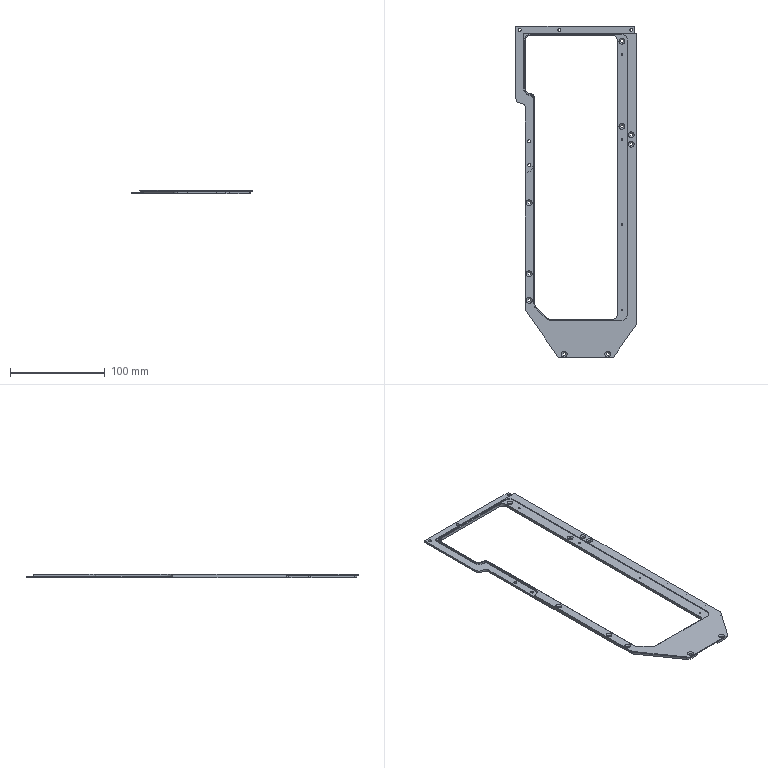NC program | NX | posted with a generic post | part box 127 x 351 x 4 mm
Whole program:
N10 G17 G21 G94 G90
(DRILL_HOLES_COPY_1 , TOOL : CHAMFER_D8-90DEG)
N12 T01 M6
N14 G53
N16 G17 G0 G90 X-111.048 Y28.911 S2500 M3
N18 G43 Z20. H1
N20 G94 G82 G98 Z-2.6 F250. P200 R3.
N22 X-61.048
N24 X-6.048
N26 X48.952
N28 X103.952
N30 X153.952
N32 Y-40.61
N34 X103.952 Y-30.61
N36 X48.952
N38 X-6.048
N40 X-61.048
N42 X-111.048
N44 G80
N46 G0 X-111.048 Y-30.61 Z20.
(PLANAR_MILL_8_1 , TOOL : CHAMFER_D8-90DEG)
N48 X-190.5 Y-67.5 S3000
N50 Z2.9
N52 G1 Z-0.1 F1000.
N54 X-182.5
N56 X182.5
N58 Y67.5
N60 Y75.5
N62 Z2.9
N64 G0 Z20.
N66 M5
(DRILL_HOLES_COPY_COPY , TOOL : DRILL_D4.3-54-83)
N68 T00 M6
N70 G53
N72 G17 G0 G90 X-111.048 Y28.911 S3000 M3
N74 G43 Z20. H0
N76 G94 G82 G98 Z-15. F200. P200 R3.
N78 X-61.048
N80 X-6.048
N82 X48.952
N84 X103.952
N86 X153.952
N88 Y-40.61
N90 X103.952 Y-30.61
N92 X48.952
N94 X-6.048
N96 X-61.048
N98 X-111.048
N100 G80
N102 G0 X-111.048 Y-30.61 Z20.
N104 M5
(DRILL_HOLES_COPY_COPY_COPY , TOOL : UPPER_ROW_M5-22-D5.5-60)
N106 M6
N108 G53
N110 G17 G0 G90 X-111.048 Y28.911 S300 M3
N112 G43 Z20. H0
N114 G84 G94 G98 Z-10. F240. R3.
N116 X-61.048
N118 X-6.048
N120 X48.952
N122 X103.952
N124 X153.952
N126 Y-40.61
N128 X103.952 Y-30.61
N130 X48.952
N132 X-6.048
N134 X-61.048
N136 X-111.048
N138 G80
N140 G0 X-111.048 Y-30.61 Z20.
N142 M5
N144 M2